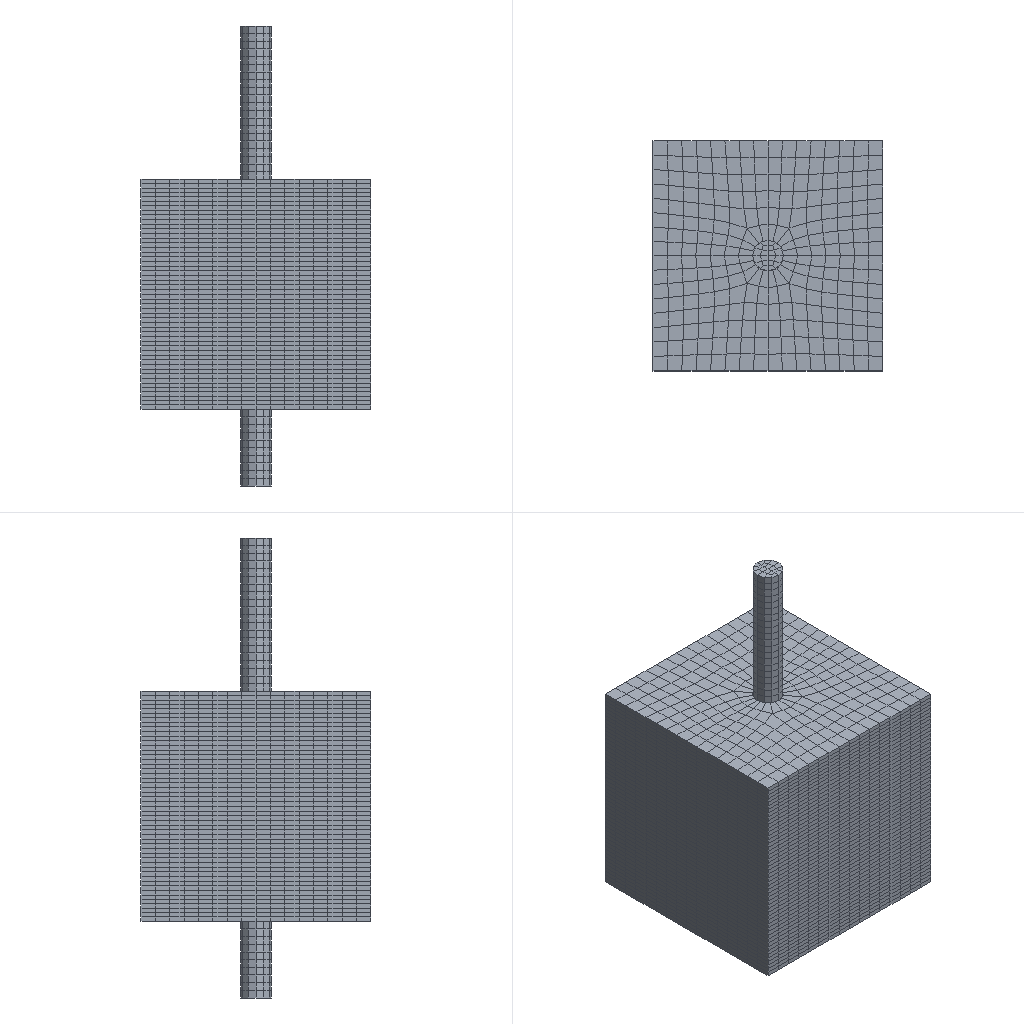Simulation study | abaqus
Set-up summary:
category,name,step,type,value,unit,region
solver,abaqus
solver,version,,,Abaqus/Standard 2020
units,not stated in the deck,,not stated
analysis,deck,,static,static
load_step,Step-1,Step-1,static,nlgeom=True
contact,interactions,,,general=0 pairs=1 ties=0
load_step,requested,,,1
mesh,nodes,,,16641
mesh,elements,,,13800
element_type,C3D8R,,solid,13800
load,load commands in deck,,count,2
bc,support commands in deck,,count,7
material,C40,,in results
material,STEEL,,in results
check,setup vs results,,match,"per instance, exact: element labels, types and connectivity; labels of the nodes the elements use; coordinates of those nodes at SINGLE_PRECISION in 2 of 2 instance(s)"
Abaqus input file, long lists of numbers shortened:
*Heading
** Job name: Job-1 Model name: Model-1
** Generated by: Abaqus/CAE 2020
*Preprint, echo=NO, model=NO, history=NO, contact=NO
**
** PARTS
**
*Part, name=b-fianl
*Node
      1,          75.,        -150.,          75.
      2,          75.,         -85.,          75.
** (14992 more lines like these left out)
*Element, type=C3D8R
   1, 1215, 1216, 6602, 6380,   66,   67, 1084, 1083
   2, 1216,   89, 1130, 6602,   67,    1,   68, 1084
** (12598 more lines like these left out)
*Nset, nset=Set-2, generate
     1,  14994,      1
*Elset, elset=Set-2, generate
     1,  12600,      1
** Section: Section-2
*Solid Section, elset=Set-2, material=c40
,
*End Part
**
*Part, name=steel
*Node
      1,         -10.,           0.,         125.
      2,           0.,           0.,         125.
** (1645 more lines like these left out)
*Element, type=C3D8R
 1,  416,  417, 1227, 1221,   36,   37,  405,  404
 2,  417,   48,  406, 1227,   37,    1,   38,  405
** (1198 more lines like these left out)
*Nset, nset=Set-1, generate
    1,  1647,     1
*Elset, elset=Set-1, generate
    1,  1200,     1
** Section: Section-1
*Solid Section, elset=Set-1, material=steel
,
*End Part
**
**
** ASSEMBLY
**
*Assembly, name=Assembly
**
*Instance, name=steel-1, part=steel
         75.,         -75.,         -50.
*End Instance
**
*Instance, name=b-fianl-1, part=b-fianl
*End Instance
**
*Node
      1,          75.,         -75.,         250.
*Nset, nset=Set-1, instance=b-fianl-1
   36,   37,   38,   39,   40,   42,   43,   44,   50,   51,   52,   53,  728,  729,  730,  731
  732,  733,  734,  735,  736,  737,  738,  739,  740,  741,  742,  743,  762,  763,  764,  765
** (17 more lines like these left out)
*Elset, elset=Set-1, instance=b-fianl-1
  7978,  7982,  7986,  7990,  7994,  7998,  8002,  8006,  8010,  8014,  8015,  8019,  8176,  8177,  8178,  8188
  8189,  8190,  8191,  8192,  8193,  8194,  8195,  8196,  8197,  8198,  8199,  8200,  8201,  8202,  8203,  8204
** (14 more lines like these left out)
*Nset, nset=Set-28
 1,
*Nset, nset=m_Set-27
 1,
*Elset, elset=_Surf-4_S3, internal, instance=b-fianl-1
     1,     2,    11,    12,    21,    22,    31,    32,    41,    42,    51,    52,    61,    62,    71,    72
    81,    82,   298,   299,   300,   301,   302,   328,   329,   330,   331,   332,   358,   359,   360,   361
** (77 more lines like these left out)
*Elset, elset=_Surf-4_S4, internal, instance=b-fianl-1
   141,   147,   153,   159,   165,   171,   177,   183,   189,   195,   201,   207,   213,   219,   225,   231
   237,   243,   249,   255,   261,   267,   273,   279,   285,   291,   297,   302,   307,   312,   317,   322
** (67 more lines like these left out)
*Elset, elset=_Surf-4_S2, internal, instance=b-fianl-1
  1810,  1811,  1812,  1813,  1814,  1815,  1816,  1817,  1818,  1819,  1820,  1821,  1822,  1823,  1824,  1825
  1826,  1827,  1828,  1829,  1830,  1831,  1832,  1833,  1834,  1835,  1836,  1837,  1838,  1839,  1840,  1841
** (51 more lines like these left out)
*Surface, type=ELEMENT, name=Surf-4
_Surf-4_S3, S3
_Surf-4_S4, S4
_Surf-4_S2, S2
*Elset, elset=_m_Surf-2_S3, internal, instance=steel-1
    1,    2,    3,    4,    5,    6,    7,    8,    9,   10,   38,   39,   40,   41,   42,   43
   44,   45,   46,   47,   48,   49,   56,   57,   58,   59,   60,   61,   62,   63,   64,   65
** (18 more lines like these left out)
*Elset, elset=_m_Surf-2_S4, internal, instance=steel-1
   21,   22,   23,   24,   25,   50,   51,   52,   53,   54,   55,   76,   77,   78,   79,   80
  111,  112,  113,  114,  115,  116,  117,  118,  119,  120,  166,  167,  168,  169,  170,  171
** (20 more lines like these left out)
*Elset, elset=_m_Surf-2_S2, internal, instance=steel-1
  105,  106,  107,  108,  109,  110,  136,  137,  138,  139,  140,  141,  142,  143,  144,  145
  146,  147,  148,  149,  150,  151,  152,  153,  215,  216,  217,  218,  219,  220,  301,  302
** (3 more lines like these left out)
*Surface, type=ELEMENT, name=m_Surf-2
_m_Surf-2_S3, S3
_m_Surf-2_S4, S4
_m_Surf-2_S2, S2
*Elset, elset=_s_Surf-1_S2, internal, instance=steel-1
 386, 387, 406, 407, 426
*Elset, elset=_s_Surf-1_S3, internal, instance=steel-1
  741,  751,  821,  831,  861, 1051, 1061, 1091
*Elset, elset=_s_Surf-1_S4, internal, instance=steel-1
  730,  740,  770,  850,  860, 1080, 1090
*Surface, type=ELEMENT, name=s_Surf-1
_s_Surf-1_S2, S2
_s_Surf-1_S3, S3
_s_Surf-1_S4, S4
*Elset, elset=_s_Surf-2_S3, internal, instance=b-fianl-1
   109,   110,   111,   112,   113,   114,   115,   116,   117,   118,   119,   120,   121,   122,   123,   124
   125,   126,   127,   128,   129,   130,   131,   132,   133,   134,   135,  1243,  1244,  1245,  1246,  1247
** (29 more lines like these left out)
*Elset, elset=_s_Surf-2_S4, internal, instance=b-fianl-1
    91,    92,    93,    94,    95,    96,    97,    98,    99,   100,   101,   102,   103,   104,   105,   106
   107,   108,   568,   569,   570,   571,   572,   573,   574,   575,   576,   577,   578,   579,   580,   581
** (22 more lines like these left out)
*Elset, elset=_s_Surf-2_S2, internal, instance=b-fianl-1
   676,   677,   678,   679,   680,   681,   682,   683,   684,   685,   686,   687,   688,   689,   690,   691
   692,   693,   694,   695,   696,   697,   698,   699,   700,   701,   702,  5212,  5213,  5214,  5215,  5216
** (7 more lines like these left out)
*Surface, type=ELEMENT, name=s_Surf-2
_s_Surf-2_S3, S3
_s_Surf-2_S4, S4
_s_Surf-2_S2, S2
** Constraint: Constraint-1
*Coupling, constraint name=Constraint-1, ref node=m_Set-27, surface=s_Surf-1
*Kinematic
*Spring, elset=Springs/Dashpots-1-spring
3, 3
1000.
*Dashpot, elset=Springs/Dashpots-1-dashpot
3, 3
100.
*Element, type=Spring2, elset=Springs/Dashpots-1-spring
1, steel-1.3, b-fianl-1.2
3, steel-1.1, b-fianl-1.3
** (2 more lines like these left out)
*Element, type=Dashpot2, elset=Springs/Dashpots-1-dashpot
2, steel-1.3, b-fianl-1.2
4, steel-1.1, b-fianl-1.3
** (2 more lines like these left out)
*Spring, elset=Springs/Dashpots-2-spring
3, 3
1000.
*Dashpot, elset=Springs/Dashpots-2-dashpot
3, 3
100.
*Element, type=Spring2, elset=Springs/Dashpots-2-spring
9, steel-1.11, b-fianl-1.8
11, steel-1.13, b-fianl-1.6
** (2 more lines like these left out)
*Element, type=Dashpot2, elset=Springs/Dashpots-2-dashpot
10, steel-1.11, b-fianl-1.8
12, steel-1.13, b-fianl-1.6
** (2 more lines like these left out)
*Spring, elset=Springs/Dashpots-3-spring
3, 3
1000.
*Dashpot, elset=Springs/Dashpots-3-dashpot
3, 3
100.
*Element, type=Spring2, elset=Springs/Dashpots-3-spring
17, steel-1.6, b-fianl-1.24
19, steel-1.5, b-fianl-1.27
** (2 more lines like these left out)
*Element, type=Dashpot2, elset=Springs/Dashpots-3-dashpot
18, steel-1.6, b-fianl-1.24
20, steel-1.5, b-fianl-1.27
** (2 more lines like these left out)
*End Assembly
*Amplitude, name=Amp-1
             0.,              0.,              1.,              1.
**
** MATERIALS
**
*Material, name=c40
*Density
 2.5e-09,
*Elastic
32500., 0.2
*Concrete Damaged Plasticity
30.,   0.1,  1.16, 0.667,  0.01
*Concrete Compression Hardening
 31.839,          0.
  35.238, 0.0001688
  37.656, 0.0002734
 39.058, 0.0004092
    39.5, 0.0005746
 38.815, 0.0007747
 37.101,  0.001006
  34.823,  0.001256
 32.332,  0.001511
 29.849,  0.001767
 27.497,  0.002018
 25.334,   0.002263
 23.376,  0.002503
 21.619,  0.002736
 20.051,  0.002963
 18.651,  0.003185
 17.402,  0.003403
 16.285,  0.003616
 15.284,  0.003826
 14.385,   0.004032
 13.573,  0.004236
 12.839,  0.004438
 12.173,  0.004637
 11.567,   0.004835
  11.013,  0.005031
*Concrete Tension Stiffening
  2.09,       0.
   2.4, 8.74e-06
  2.67, 1.23e-05
  2.86, 1.81e-05
  2.94, 2.75e-05
   2.8, 4.37e-05
  2.55, 6.31e-05
   2.3, 8.27e-05
  2.07, 0.000102
  1.86,  0.00012
  1.69, 0.000137
  1.55, 0.000153
  1.42, 0.000169
  1.31, 0.000184
  1.22, 0.000198
  1.14, 0.000213
  1.07, 0.000227
  1.01,  0.00024
 0.956, 0.000254
 0.908, 0.000267
 0.864,  0.00028
 0.825, 0.000293
 0.789, 0.000306
 0.757, 0.000319
 0.727, 0.000332
*Concrete Compression Damage
        0.,          0.
 0.06977, 0.0001688
  0.1005, 0.0002734
  0.1363, 0.0004092
  0.176, 0.0005746
  0.2212, 0.0007747
  0.271,  0.001006
  0.3214,  0.001256
  0.3699,  0.001511
  0.4151,  0.001767
  0.4565,  0.002018
  0.4939,   0.002263
  0.5275,  0.002503
   0.5577,  0.002736
  0.5849,  0.002963
   0.6093,  0.003185
  0.6313,  0.003403
  0.6511,  0.003616
  0.6691,  0.003826
  0.6855,   0.004032
  0.7004,  0.004236
  0.7141,  0.004438
  0.7266,  0.004637
  0.7382,   0.004835
  0.7488,  0.005031
  0.7586,  0.005226
  0.7678,  0.005419
  0.7763,  0.005611
  0.7842,  0.005802
  0.7915,  0.005993
  0.7984,  0.006182
  0.8049,  0.006371
  0.811,  0.006559
  0.8167,  0.006747
  0.8221,  0.006933
  0.8627,  0.008781
  0.8884,   0.01061
  0.906,   0.01242
  0.9188,   0.01423
  0.9286,   0.01603
** (21 more lines like these left out)
*Concrete Tension Damage, compression recovery=0.45
     0.,       0.
 0.0544, 8.74e-06
 0.0674, 1.23e-05
 0.0893, 1.81e-05
  0.124, 2.75e-05
  0.186, 4.37e-05
  0.255, 6.31e-05
  0.321, 8.27e-05
   0.38, 0.000102
  0.431,  0.00012
  0.475, 0.000137
  0.513, 0.000153
  0.546, 0.000169
  0.575, 0.000184
  0.601, 0.000198
  0.623, 0.000213
  0.643, 0.000227
  0.661,  0.00024
  0.678, 0.000254
  0.692, 0.000267
  0.706,  0.00028
  0.718, 0.000293
  0.729, 0.000306
  0.739, 0.000319
  0.749, 0.000332
  0.757, 0.000344
  0.765, 0.000357
  0.773, 0.000369
   0.78, 0.000382
  0.787, 0.000394
  0.793, 0.000407
  0.799, 0.000419
  0.804, 0.000431
  0.809, 0.000443
  0.814, 0.000456
  0.851, 0.000577
  0.875, 0.000697
  0.892, 0.000816
  0.905, 0.000935
  0.915,  0.00105
** (31 more lines like these left out)
*Material, name=steel
*Density
 7.85e-09,
*Elastic
210000., 0.3
*Plastic
296.,     0.
360., 0.0015
**
** INTERACTION PROPERTIES
**
*Surface Interaction, name=IntProp-1
1.,
*Friction, slip tolerance=0.005
 0.15,
*Surface Behavior, pressure-overclosure=HARD
**
** INTERACTIONS
**
** Interaction: Int-1
*Contact Pair, interaction=IntProp-1, type=SURFACE TO SURFACE
s_Surf-2, m_Surf-2
** ----------------------------------------------------------------
**
** STEP: Step-1
**
*Step, name=Step-1, nlgeom=YES, inc=1000
*Static, stabilize=0.0002, allsdtol=0.05, continue=NO
0.01, 1., 1e-05, 0.1
**
** BOUNDARY CONDITIONS
**
** Name: BC-1 Type: 对称/反对称/完全固定
*Boundary
Set-1, ENCASTRE
** Name: [REDACTED] : Displacement/rotation angle
*Boundary, amplitude=Amp-1
Set-28, 1, 1
Set-28, 2, 2
Set-28, 3, 3, 5.
Set-28, 4, 4
Set-28, 5, 5
Set-28, 6, 6
**
** LOADS
**
** Name: Load-1   Type: Pressure
*Dsload
Surf-4, P, 3.6
**
** OUTPUT REQUESTS
**
*Restart, write, frequency=0
**
** FIELD OUTPUT: F-Output-1
**
*Output, field
*Node Output
CF, RF, RM, RT, TF, U, V
*Element Output, directions=YES
DAMAGEC, DAMAGET, E, LE, MISES, MISESMAX, MISESONLY, P, PE, PEEQ, PEEQMAX, PEEQT, PEMAG, PRESSONLY, S, SDEG
SEQUT, SF, SSAVG, YIELDPOT
*Contact Output
CDISP, CDSTRESS, CFORCE, CNAREA, CSTATUS, CSTRESS, CSTRESSETOS, PPRESS
**
** HISTORY OUTPUT: H-Output-1
**
*Output, history, variable=PRESELECT
*End Step
Results summary:
result,step,,completed,increments=102 time=1.0/1.0
result,analysis,,,static
result,last_loadstep,,,1
result,analysis steps,,count,1
result,primary field,,,U
result,reaction total,,FX,-0.03106,model units
result,reaction total,,FY,-0.000725,model units
result,reaction total,,FZ,-7.489,model units